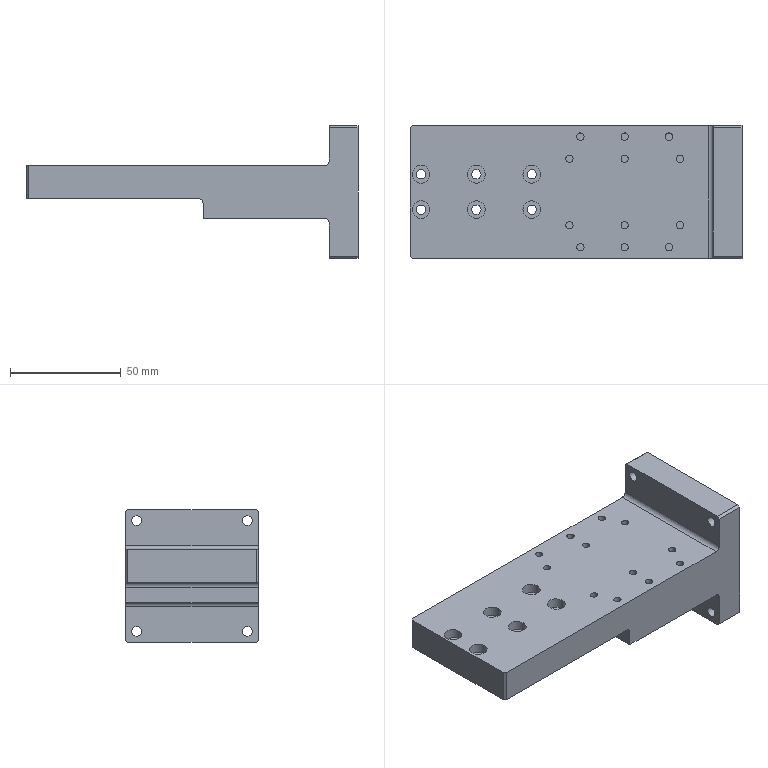Part | 1 solid | 75 faces | box 150 x 60 x 60 mm | volume 196633 mm3 | plane 40 | cylinder 35 | commonest cylinder face diameters 3.3 x16 4.2 x6 8 x6 4.5 x4 4 x3